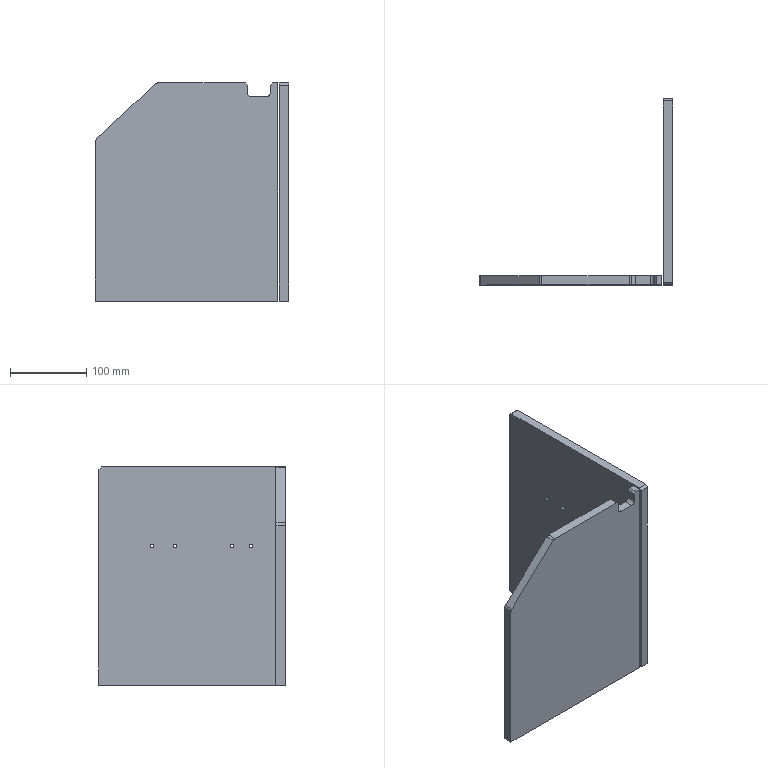Part | SolidWorks | features Cut 3, Fillet 3, HoleWzd 3, Chamfer 2, Extrusion 1 | 2 solids | 57 faces | box 254 x 245 x 287 mm | volume 1625619 mm3 | cylinder 24 | plane 21 | cone 12 | commonest cylinder face diameters 4.2 x12 5 x8 10 x4